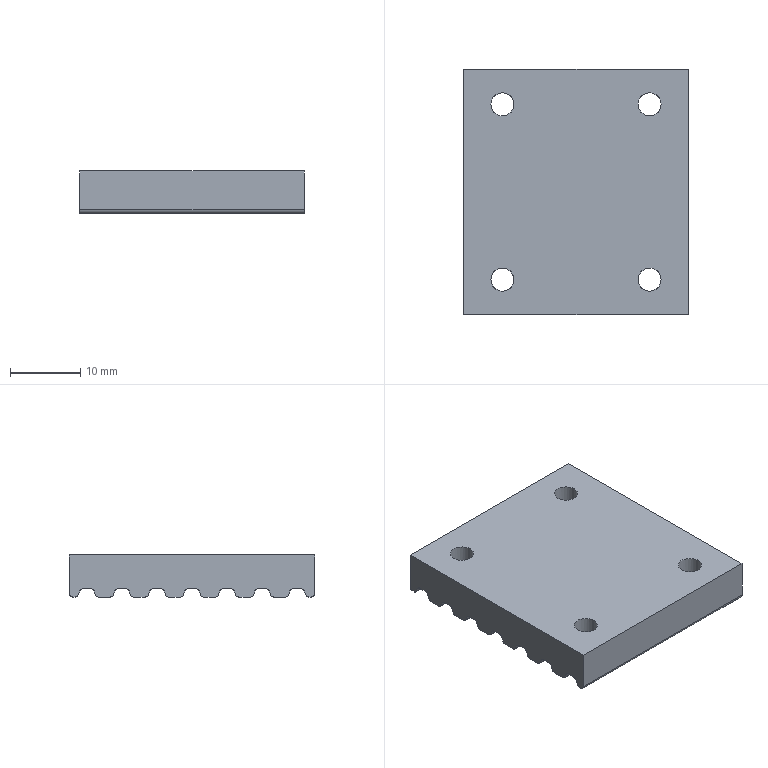Part | NX | 1 solid | 88 faces | box 32 x 35 x 6 mm | volume 5914 mm3 | plane 46 | cylinder 42 | commonest cylinder face diameters 1 x38 3.3 x4